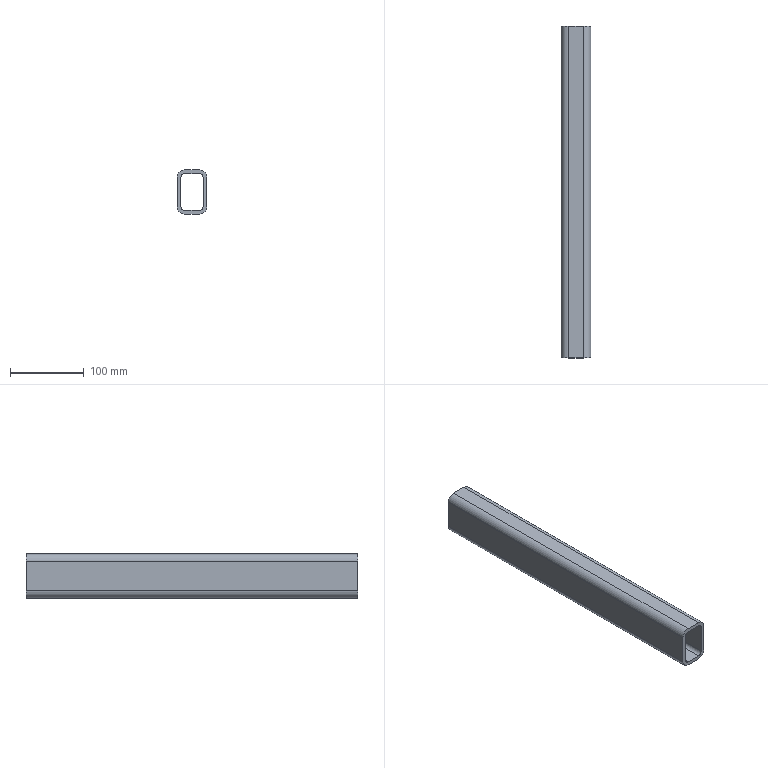Part | STEP file | HL4GD-1.30.110 base frame rear crossmember--20251212 | 1 solid | 18 faces | box 40 x 450 x 60 mm | volume 376029 mm3 | plane 10 | cylinder 8 | commonest cylinder face diameters 10 x4 20 x4
STEP:
#1=CARTESIAN_POINT('',(0.,0.,0.));
#2=DIRECTION('',(0.,0.,1.));
#3=DIRECTION('',(1.,0.,0.));
#4=AXIS2_PLACEMENT_3D('',#1,#2,#3);
#5=CARTESIAN_POINT('',(1525.,1110.,410.));
#6=VERTEX_POINT('',#5);
#7=CARTESIAN_POINT('',(1520.,1110.,415.));
#8=VERTEX_POINT('',#7);
#9=CARTESIAN_POINT('',(1525.,1110.,415.));
#10=DIRECTION('',(0.,1.,0.));
#11=DIRECTION('',(0.,0.,1.));
#12=AXIS2_PLACEMENT_3D('',#9,#10,#11);
#13=CIRCLE('',#12,5.);
#14=CARTESIAN_POINT('',(1525.,530.,415.));
#15=DIRECTION('',(0.,1.,0.));
#16=DIRECTION('',(-1.,0.,0.));
#17=AXIS2_PLACEMENT_3D('',#14,#15,#16);
#18=CYLINDRICAL_SURFACE('',#17,5.);
#19=CARTESIAN_POINT('',(1.571,580.));
#20=DIRECTION('',(1.,0.));
#21=VECTOR('',#20,1.);
#22=LINE('',#19,#21);
#23=(GEOMETRIC_REPRESENTATION_CONTEXT(2)PARAMETRIC_REPRESENTATION_CONTEXT()REPRESENTATION_CONTEXT('',''));
#24=DEFINITIONAL_REPRESENTATION('',(#22),#23);
#25=PCURVE('',#18,#24);
#26=CARTESIAN_POINT('',(2045.,1110.,435.));
#27=DIRECTION('',(0.,1.,0.));
#28=DIRECTION('',(0.,0.,1.));
#29=AXIS2_PLACEMENT_3D('',#26,#27,#28);
#30=PLANE('',#29);
#31=CARTESIAN_POINT('',(-20.,-520.));
#32=DIRECTION('',(1.,0.));
#33=AXIS2_PLACEMENT_2D('',#31,#32);
#34=CIRCLE('',#33,5.);
#35=(GEOMETRIC_REPRESENTATION_CONTEXT(2)PARAMETRIC_REPRESENTATION_CONTEXT()REPRESENTATION_CONTEXT('',''));
#36=DEFINITIONAL_REPRESENTATION('',(#34),#35);
#37=PCURVE('',#30,#36);
#38=SURFACE_CURVE('',#13,(#25,#37),.PCURVE_S1.);
#39=EDGE_CURVE('',#6,#8,#38,.T.);
#40=ORIENTED_EDGE('',*,*,#39,.F.);
#41=CARTESIAN_POINT('',(1525.,660.,410.));
#42=VERTEX_POINT('',#41);
#43=CARTESIAN_POINT('',(1525.,530.,410.));
#44=DIRECTION('',(0.,1.,0.));
#45=VECTOR('',#44,1.);
#46=LINE('',#43,#45);
#47=CARTESIAN_POINT('',(4.712,0.));
#48=DIRECTION('',(0.,1.));
#49=VECTOR('',#48,1.);
#50=LINE('',#47,#49);
#51=(GEOMETRIC_REPRESENTATION_CONTEXT(2)PARAMETRIC_REPRESENTATION_CONTEXT()REPRESENTATION_CONTEXT('',''));
#52=DEFINITIONAL_REPRESENTATION('',(#50),#51);
#53=PCURVE('',#18,#52);
#54=CARTESIAN_POINT('',(1545.,530.,410.));
#55=DIRECTION('',(0.,0.,1.));
#56=DIRECTION('',(1.,0.,0.));
#57=AXIS2_PLACEMENT_3D('',#54,#55,#56);
#58=PLANE('',#57);
#59=CARTESIAN_POINT('',(-20.,0.));
#60=DIRECTION('',(0.,1.));
#61=VECTOR('',#60,1.);
#62=LINE('',#59,#61);
#63=(GEOMETRIC_REPRESENTATION_CONTEXT(2)PARAMETRIC_REPRESENTATION_CONTEXT()REPRESENTATION_CONTEXT('',''));
#64=DEFINITIONAL_REPRESENTATION('',(#62),#63);
#65=PCURVE('',#58,#64);
#66=SURFACE_CURVE('',#46,(#53,#65),.PCURVE_S1.);
#67=EDGE_CURVE('',#42,#6,#66,.T.);
#68=ORIENTED_EDGE('',*,*,#67,.F.);
#69=CARTESIAN_POINT('',(1520.,660.,415.));
#70=VERTEX_POINT('',#69);
#71=CARTESIAN_POINT('',(1525.,660.,415.));
#72=DIRECTION('',(0.,-1.,0.));
#73=DIRECTION('',(0.,0.,-1.));
#74=AXIS2_PLACEMENT_3D('',#71,#72,#73);
#75=CIRCLE('',#74,5.);
#76=CARTESIAN_POINT('',(10.996,130.));
#77=DIRECTION('',(-1.,0.));
#78=VECTOR('',#77,1.);
#79=LINE('',#76,#78);
#80=(GEOMETRIC_REPRESENTATION_CONTEXT(2)PARAMETRIC_REPRESENTATION_CONTEXT()REPRESENTATION_CONTEXT('',''));
#81=DEFINITIONAL_REPRESENTATION('',(#79),#80);
#82=PCURVE('',#18,#81);
#83=CARTESIAN_POINT('',(1555.,660.,412.726));
#84=DIRECTION('',(0.,-1.,0.));
#85=DIRECTION('',(0.,0.,-1.));
#86=AXIS2_PLACEMENT_3D('',#83,#84,#85);
#87=PLANE('',#86);
#88=CARTESIAN_POINT('',(-2.274,-30.));
#89=DIRECTION('',(1.,0.));
#90=AXIS2_PLACEMENT_2D('',#88,#89);
#91=CIRCLE('',#90,5.);
#92=(GEOMETRIC_REPRESENTATION_CONTEXT(2)PARAMETRIC_REPRESENTATION_CONTEXT()REPRESENTATION_CONTEXT('',''));
#93=DEFINITIONAL_REPRESENTATION('',(#91),#92);
#94=PCURVE('',#87,#93);
#95=SURFACE_CURVE('',#75,(#82,#94),.PCURVE_S1.);
#96=EDGE_CURVE('',#70,#42,#95,.T.);
#97=ORIENTED_EDGE('',*,*,#96,.F.);
#98=CARTESIAN_POINT('',(1520.,530.,415.));
#99=DIRECTION('',(0.,1.,0.));
#100=VECTOR('',#99,1.);
#101=LINE('',#98,#100);
#102=CARTESIAN_POINT('',(6.283,0.));
#103=DIRECTION('',(0.,1.));
#104=VECTOR('',#103,1.);
#105=LINE('',#102,#104);
#106=(GEOMETRIC_REPRESENTATION_CONTEXT(2)PARAMETRIC_REPRESENTATION_CONTEXT()REPRESENTATION_CONTEXT('',''));
#107=DEFINITIONAL_REPRESENTATION('',(#105),#106);
#108=PCURVE('',#18,#107);
#109=CARTESIAN_POINT('',(1520.,530.,415.));
#110=DIRECTION('',(1.,0.,0.));
#111=DIRECTION('',(0.,0.,-1.));
#112=AXIS2_PLACEMENT_3D('',#109,#110,#111);
#113=PLANE('',#112);
#114=CARTESIAN_POINT('',(0.,0.));
#115=DIRECTION('',(0.,1.));
#116=VECTOR('',#115,1.);
#117=LINE('',#114,#116);
#118=(GEOMETRIC_REPRESENTATION_CONTEXT(2)PARAMETRIC_REPRESENTATION_CONTEXT()REPRESENTATION_CONTEXT('',''));
#119=DEFINITIONAL_REPRESENTATION('',(#117),#118);
#120=PCURVE('',#113,#119);
#121=SURFACE_CURVE('',#101,(#108,#120),.PCURVE_S1.);
#122=EDGE_CURVE('',#70,#8,#121,.T.);
#123=ORIENTED_EDGE('',*,*,#122,.T.);
#124=EDGE_LOOP('',(#40,#68,#97,#123));
#125=FACE_BOUND('',#124,.F.);
#126=ADVANCED_FACE('',(#125),#18,.F.);
#127=ORIENTED_EDGE('',*,*,#67,.F.);
#128=CARTESIAN_POINT('',(1545.,660.,410.));
#129=VERTEX_POINT('',#128);
#130=CARTESIAN_POINT('',(1545.,660.,410.));
#131=DIRECTION('',(1.,0.,0.));
#132=VECTOR('',#131,1.);
#133=LINE('',#130,#132);
#134=CARTESIAN_POINT('',(0.,130.));
#135=DIRECTION('',(1.,0.));
#136=VECTOR('',#135,1.);
#137=LINE('',#134,#136);
#138=(GEOMETRIC_REPRESENTATION_CONTEXT(2)PARAMETRIC_REPRESENTATION_CONTEXT()REPRESENTATION_CONTEXT('',''));
#139=DEFINITIONAL_REPRESENTATION('',(#137),#138);
#140=PCURVE('',#58,#139);
#141=CARTESIAN_POINT('',(2.726,-10.));
#142=DIRECTION('',(0.,1.));
#143=VECTOR('',#142,1.);
#144=LINE('',#141,#143);
#145=(GEOMETRIC_REPRESENTATION_CONTEXT(2)PARAMETRIC_REPRESENTATION_CONTEXT()REPRESENTATION_CONTEXT('',''));
#146=DEFINITIONAL_REPRESENTATION('',(#144),#145);
#147=PCURVE('',#87,#146);
#148=SURFACE_CURVE('',#133,(#140,#147),.PCURVE_S1.);
#149=EDGE_CURVE('',#42,#129,#148,.T.);
#150=ORIENTED_EDGE('',*,*,#149,.T.);
#151=CARTESIAN_POINT('',(1545.,1110.,410.));
#152=VERTEX_POINT('',#151);
#153=CARTESIAN_POINT('',(1545.,530.,410.));
#154=DIRECTION('',(0.,1.,0.));
#155=VECTOR('',#154,1.);
#156=LINE('',#153,#155);
#157=CARTESIAN_POINT('',(0.,0.));
#158=DIRECTION('',(0.,1.));
#159=VECTOR('',#158,1.);
#160=LINE('',#157,#159);
#161=(GEOMETRIC_REPRESENTATION_CONTEXT(2)PARAMETRIC_REPRESENTATION_CONTEXT()REPRESENTATION_CONTEXT('',''));
#162=DEFINITIONAL_REPRESENTATION('',(#160),#161);
#163=PCURVE('',#58,#162);
#164=CARTESIAN_POINT('',(1545.,530.,415.));
#165=DIRECTION('',(0.,1.,0.));
#166=DIRECTION('',(-1.,0.,0.));
#167=AXIS2_PLACEMENT_3D('',#164,#165,#166);
#168=CYLINDRICAL_SURFACE('',#167,5.);
#169=CARTESIAN_POINT('',(4.712,0.));
#170=DIRECTION('',(0.,1.));
#171=VECTOR('',#170,1.);
#172=LINE('',#169,#171);
#173=(GEOMETRIC_REPRESENTATION_CONTEXT(2)PARAMETRIC_REPRESENTATION_CONTEXT()REPRESENTATION_CONTEXT('',''));
#174=DEFINITIONAL_REPRESENTATION('',(#172),#173);
#175=PCURVE('',#168,#174);
#176=SURFACE_CURVE('',#156,(#163,#175),.PCURVE_S1.);
#177=EDGE_CURVE('',#129,#152,#176,.T.);
#178=ORIENTED_EDGE('',*,*,#177,.T.);
#179=CARTESIAN_POINT('',(1545.,1110.,410.));
#180=DIRECTION('',(-1.,0.,0.));
#181=VECTOR('',#180,1.);
#182=LINE('',#179,#181);
#183=CARTESIAN_POINT('',(0.,580.));
#184=DIRECTION('',(-1.,0.));
#185=VECTOR('',#184,1.);
#186=LINE('',#183,#185);
#187=(GEOMETRIC_REPRESENTATION_CONTEXT(2)PARAMETRIC_REPRESENTATION_CONTEXT()REPRESENTATION_CONTEXT('',''));
#188=DEFINITIONAL_REPRESENTATION('',(#186),#187);
#189=PCURVE('',#58,#188);
#190=CARTESIAN_POINT('',(-25.,-500.));
#191=DIRECTION('',(0.,-1.));
#192=VECTOR('',#191,1.);
#193=LINE('',#190,#192);
#194=(GEOMETRIC_REPRESENTATION_CONTEXT(2)PARAMETRIC_REPRESENTATION_CONTEXT()REPRESENTATION_CONTEXT('',''));
#195=DEFINITIONAL_REPRESENTATION('',(#193),#194);
#196=PCURVE('',#30,#195);
#197=SURFACE_CURVE('',#182,(#189,#196),.PCURVE_S1.);
#198=EDGE_CURVE('',#152,#6,#197,.T.);
#199=ORIENTED_EDGE('',*,*,#198,.T.);
#200=EDGE_LOOP('',(#127,#150,#178,#199));
#201=FACE_BOUND('',#200,.T.);
#202=ADVANCED_FACE('',(#201),#58,.T.);
#203=CARTESIAN_POINT('',(1550.,1110.,415.));
#204=VERTEX_POINT('',#203);
#205=CARTESIAN_POINT('',(1545.,1110.,415.));
#206=DIRECTION('',(0.,1.,0.));
#207=DIRECTION('',(0.,0.,1.));
#208=AXIS2_PLACEMENT_3D('',#205,#206,#207);
#209=CIRCLE('',#208,5.);
#210=CARTESIAN_POINT('',(1.571,580.));
#211=DIRECTION('',(1.,0.));
#212=VECTOR('',#211,1.);
#213=LINE('',#210,#212);
#214=(GEOMETRIC_REPRESENTATION_CONTEXT(2)PARAMETRIC_REPRESENTATION_CONTEXT()REPRESENTATION_CONTEXT('',''));
#215=DEFINITIONAL_REPRESENTATION('',(#213),#214);
#216=PCURVE('',#168,#215);
#217=CARTESIAN_POINT('',(-20.,-500.));
#218=DIRECTION('',(1.,0.));
#219=AXIS2_PLACEMENT_2D('',#217,#218);
#220=CIRCLE('',#219,5.);
#221=(GEOMETRIC_REPRESENTATION_CONTEXT(2)PARAMETRIC_REPRESENTATION_CONTEXT()REPRESENTATION_CONTEXT('',''));
#222=DEFINITIONAL_REPRESENTATION('',(#220),#221);
#223=PCURVE('',#30,#222);
#224=SURFACE_CURVE('',#209,(#216,#223),.PCURVE_S1.);
#225=EDGE_CURVE('',#204,#152,#224,.T.);
#226=ORIENTED_EDGE('',*,*,#225,.F.);
#227=CARTESIAN_POINT('',(1550.,660.,415.));
#228=VERTEX_POINT('',#227);
#229=CARTESIAN_POINT('',(1550.,530.,415.));
#230=DIRECTION('',(0.,1.,0.));
#231=VECTOR('',#230,1.);
#232=LINE('',#229,#231);
#233=CARTESIAN_POINT('',(3.142,0.));
#234=DIRECTION('',(0.,1.));
#235=VECTOR('',#234,1.);
#236=LINE('',#233,#235);
#237=(GEOMETRIC_REPRESENTATION_CONTEXT(2)PARAMETRIC_REPRESENTATION_CONTEXT()REPRESENTATION_CONTEXT('',''));
#238=DEFINITIONAL_REPRESENTATION('',(#236),#237);
#239=PCURVE('',#168,#238);
#240=CARTESIAN_POINT('',(1550.,530.,455.));
#241=DIRECTION('',(-1.,0.,0.));
#242=DIRECTION('',(0.,0.,1.));
#243=AXIS2_PLACEMENT_3D('',#240,#241,#242);
#244=PLANE('',#243);
#245=CARTESIAN_POINT('',(-40.,0.));
#246=DIRECTION('',(0.,1.));
#247=VECTOR('',#246,1.);
#248=LINE('',#245,#247);
#249=(GEOMETRIC_REPRESENTATION_CONTEXT(2)PARAMETRIC_REPRESENTATION_CONTEXT()REPRESENTATION_CONTEXT('',''));
#250=DEFINITIONAL_REPRESENTATION('',(#248),#249);
#251=PCURVE('',#244,#250);
#252=SURFACE_CURVE('',#232,(#239,#251),.PCURVE_S1.);
#253=EDGE_CURVE('',#228,#204,#252,.T.);
#254=ORIENTED_EDGE('',*,*,#253,.F.);
#255=CARTESIAN_POINT('',(1545.,660.,415.));
#256=DIRECTION('',(0.,-1.,0.));
#257=DIRECTION('',(0.,0.,-1.));
#258=AXIS2_PLACEMENT_3D('',#255,#256,#257);
#259=CIRCLE('',#258,5.);
#260=CARTESIAN_POINT('',(4.712,130.));
#261=DIRECTION('',(-1.,0.));
#262=VECTOR('',#261,1.);
#263=LINE('',#260,#262);
#264=(GEOMETRIC_REPRESENTATION_CONTEXT(2)PARAMETRIC_REPRESENTATION_CONTEXT()REPRESENTATION_CONTEXT('',''));
#265=DEFINITIONAL_REPRESENTATION('',(#263),#264);
#266=PCURVE('',#168,#265);
#267=CARTESIAN_POINT('',(-2.274,-10.));
#268=DIRECTION('',(1.,0.));
#269=AXIS2_PLACEMENT_2D('',#267,#268);
#270=CIRCLE('',#269,5.);
#271=(GEOMETRIC_REPRESENTATION_CONTEXT(2)PARAMETRIC_REPRESENTATION_CONTEXT()REPRESENTATION_CONTEXT('',''));
#272=DEFINITIONAL_REPRESENTATION('',(#270),#271);
#273=PCURVE('',#87,#272);
#274=SURFACE_CURVE('',#259,(#266,#273),.PCURVE_S1.);
#275=EDGE_CURVE('',#129,#228,#274,.T.);
#276=ORIENTED_EDGE('',*,*,#275,.F.);
#277=ORIENTED_EDGE('',*,*,#177,.T.);
#278=EDGE_LOOP('',(#226,#254,#276,#277));
#279=FACE_BOUND('',#278,.F.);
#280=ADVANCED_FACE('',(#279),#168,.F.);
#281=ORIENTED_EDGE('',*,*,#253,.F.);
#282=CARTESIAN_POINT('',(1550.,660.,455.));
#283=VERTEX_POINT('',#282);
#284=CARTESIAN_POINT('',(1550.,660.,455.));
#285=DIRECTION('',(0.,0.,1.));
#286=VECTOR('',#285,1.);
#287=LINE('',#284,#286);
#288=CARTESIAN_POINT('',(0.,130.));
#289=DIRECTION('',(1.,0.));
#290=VECTOR('',#289,1.);
#291=LINE('',#288,#290);
#292=(GEOMETRIC_REPRESENTATION_CONTEXT(2)PARAMETRIC_REPRESENTATION_CONTEXT()REPRESENTATION_CONTEXT('',''));
#293=DEFINITIONAL_REPRESENTATION('',(#291),#292);
#294=PCURVE('',#244,#293);
#295=CARTESIAN_POINT('',(-42.274,-5.));
#296=DIRECTION('',(-1.,0.));
#297=VECTOR('',#296,1.);
#298=LINE('',#295,#297);
#299=(GEOMETRIC_REPRESENTATION_CONTEXT(2)PARAMETRIC_REPRESENTATION_CONTEXT()REPRESENTATION_CONTEXT('',''));
#300=DEFINITIONAL_REPRESENTATION('',(#298),#299);
#301=PCURVE('',#87,#300);
#302=SURFACE_CURVE('',#287,(#294,#301),.PCURVE_S1.);
#303=EDGE_CURVE('',#228,#283,#302,.T.);
#304=ORIENTED_EDGE('',*,*,#303,.T.);
#305=CARTESIAN_POINT('',(1550.,1110.,455.));
#306=VERTEX_POINT('',#305);
#307=CARTESIAN_POINT('',(1550.,530.,455.));
#308=DIRECTION('',(0.,1.,0.));
#309=VECTOR('',#308,1.);
#310=LINE('',#307,#309);
#311=CARTESIAN_POINT('',(0.,0.));
#312=DIRECTION('',(0.,1.));
#313=VECTOR('',#312,1.);
#314=LINE('',#311,#313);
#315=(GEOMETRIC_REPRESENTATION_CONTEXT(2)PARAMETRIC_REPRESENTATION_CONTEXT()REPRESENTATION_CONTEXT('',''));
#316=DEFINITIONAL_REPRESENTATION('',(#314),#315);
#317=PCURVE('',#244,#316);
#318=CARTESIAN_POINT('',(1545.,530.,455.));
#319=DIRECTION('',(0.,1.,0.));
#320=DIRECTION('',(-1.,0.,0.));
#321=AXIS2_PLACEMENT_3D('',#318,#319,#320);
#322=CYLINDRICAL_SURFACE('',#321,5.);
#323=CARTESIAN_POINT('',(3.142,0.));
#324=DIRECTION('',(0.,1.));
#325=VECTOR('',#324,1.);
#326=LINE('',#323,#325);
#327=(GEOMETRIC_REPRESENTATION_CONTEXT(2)PARAMETRIC_REPRESENTATION_CONTEXT()REPRESENTATION_CONTEXT('',''));
#328=DEFINITIONAL_REPRESENTATION('',(#326),#327);
#329=PCURVE('',#322,#328);
#330=SURFACE_CURVE('',#310,(#317,#329),.PCURVE_S1.);
#331=EDGE_CURVE('',#283,#306,#330,.T.);
#332=ORIENTED_EDGE('',*,*,#331,.T.);
#333=CARTESIAN_POINT('',(1550.,1110.,455.));
#334=DIRECTION('',(0.,0.,-1.));
#335=VECTOR('',#334,1.);
#336=LINE('',#333,#335);
#337=CARTESIAN_POINT('',(0.,580.));
#338=DIRECTION('',(-1.,0.));
#339=VECTOR('',#338,1.);
#340=LINE('',#337,#339);
#341=(GEOMETRIC_REPRESENTATION_CONTEXT(2)PARAMETRIC_REPRESENTATION_CONTEXT()REPRESENTATION_CONTEXT('',''));
#342=DEFINITIONAL_REPRESENTATION('',(#340),#341);
#343=PCURVE('',#244,#342);
#344=CARTESIAN_POINT('',(20.,-495.));
#345=DIRECTION('',(-1.,0.));
#346=VECTOR('',#345,1.);
#347=LINE('',#344,#346);
#348=(GEOMETRIC_REPRESENTATION_CONTEXT(2)PARAMETRIC_REPRESENTATION_CONTEXT()REPRESENTATION_CONTEXT('',''));
#349=DEFINITIONAL_REPRESENTATION('',(#347),#348);
#350=PCURVE('',#30,#349);
#351=SURFACE_CURVE('',#336,(#343,#350),.PCURVE_S1.);
#352=EDGE_CURVE('',#306,#204,#351,.T.);
#353=ORIENTED_EDGE('',*,*,#352,.T.);
#354=EDGE_LOOP('',(#281,#304,#332,#353));
#355=FACE_BOUND('',#354,.T.);
#356=ADVANCED_FACE('',(#355),#244,.T.);
#357=CARTESIAN_POINT('',(1545.,1110.,460.));
#358=VERTEX_POINT('',#357);
#359=CARTESIAN_POINT('',(1545.,1110.,455.));
#360=DIRECTION('',(0.,1.,0.));
#361=DIRECTION('',(0.,0.,1.));
#362=AXIS2_PLACEMENT_3D('',#359,#360,#361);
#363=CIRCLE('',#362,5.);
#364=CARTESIAN_POINT('',(1.571,580.));
#365=DIRECTION('',(1.,0.));
#366=VECTOR('',#365,1.);
#367=LINE('',#364,#366);
#368=(GEOMETRIC_REPRESENTATION_CONTEXT(2)PARAMETRIC_REPRESENTATION_CONTEXT()REPRESENTATION_CONTEXT('',''));
#369=DEFINITIONAL_REPRESENTATION('',(#367),#368);
#370=PCURVE('',#322,#369);
#371=CARTESIAN_POINT('',(20.,-500.));
#372=DIRECTION('',(1.,0.));
#373=AXIS2_PLACEMENT_2D('',#371,#372);
#374=CIRCLE('',#373,5.);
#375=(GEOMETRIC_REPRESENTATION_CONTEXT(2)PARAMETRIC_REPRESENTATION_CONTEXT()REPRESENTATION_CONTEXT('',''));
#376=DEFINITIONAL_REPRESENTATION('',(#374),#375);
#377=PCURVE('',#30,#376);
#378=SURFACE_CURVE('',#363,(#370,#377),.PCURVE_S1.);
#379=EDGE_CURVE('',#358,#306,#378,.T.);
#380=ORIENTED_EDGE('',*,*,#379,.F.);
#381=CARTESIAN_POINT('',(1545.,660.,460.));
#382=VERTEX_POINT('',#381);
#383=CARTESIAN_POINT('',(1545.,530.,460.));
#384=DIRECTION('',(0.,1.,0.));
#385=VECTOR('',#384,1.);
#386=LINE('',#383,#385);
#387=CARTESIAN_POINT('',(1.571,0.));
#388=DIRECTION('',(0.,1.));
#389=VECTOR('',#388,1.);
#390=LINE('',#387,#389);
#391=(GEOMETRIC_REPRESENTATION_CONTEXT(2)PARAMETRIC_REPRESENTATION_CONTEXT()REPRESENTATION_CONTEXT('',''));
#392=DEFINITIONAL_REPRESENTATION('',(#390),#391);
#393=PCURVE('',#322,#392);
#394=CARTESIAN_POINT('',(1525.,530.,460.));
#395=DIRECTION('',(0.,0.,-1.));
#396=DIRECTION('',(-1.,0.,0.));
#397=AXIS2_PLACEMENT_3D('',#394,#395,#396);
#398=PLANE('',#397);
#399=CARTESIAN_POINT('',(-20.,0.));
#400=DIRECTION('',(0.,1.));
#401=VECTOR('',#400,1.);
#402=LINE('',#399,#401);
#403=(GEOMETRIC_REPRESENTATION_CONTEXT(2)PARAMETRIC_REPRESENTATION_CONTEXT()REPRESENTATION_CONTEXT('',''));
#404=DEFINITIONAL_REPRESENTATION('',(#402),#403);
#405=PCURVE('',#398,#404);
#406=SURFACE_CURVE('',#386,(#393,#405),.PCURVE_S1.);
#407=EDGE_CURVE('',#382,#358,#406,.T.);
#408=ORIENTED_EDGE('',*,*,#407,.F.);
#409=CARTESIAN_POINT('',(1545.,660.,455.));
#410=DIRECTION('',(0.,-1.,0.));
#411=DIRECTION('',(0.,0.,-1.));
#412=AXIS2_PLACEMENT_3D('',#409,#410,#411);
#413=CIRCLE('',#412,5.);
#414=CARTESIAN_POINT('',(4.712,130.));
#415=DIRECTION('',(-1.,0.));
#416=VECTOR('',#415,1.);
#417=LINE('',#414,#416);
#418=(GEOMETRIC_REPRESENTATION_CONTEXT(2)PARAMETRIC_REPRESENTATION_CONTEXT()REPRESENTATION_CONTEXT('',''));
#419=DEFINITIONAL_REPRESENTATION('',(#417),#418);
#420=PCURVE('',#322,#419);
#421=CARTESIAN_POINT('',(-42.274,-10.));
#422=DIRECTION('',(1.,0.));
#423=AXIS2_PLACEMENT_2D('',#421,#422);
#424=CIRCLE('',#423,5.);
#425=(GEOMETRIC_REPRESENTATION_CONTEXT(2)PARAMETRIC_REPRESENTATION_CONTEXT()REPRESENTATION_CONTEXT('',''));
#426=DEFINITIONAL_REPRESENTATION('',(#424),#425);
#427=PCURVE('',#87,#426);
#428=SURFACE_CURVE('',#413,(#420,#427),.PCURVE_S1.);
#429=EDGE_CURVE('',#283,#382,#428,.T.);
#430=ORIENTED_EDGE('',*,*,#429,.F.);
#431=ORIENTED_EDGE('',*,*,#331,.T.);
#432=EDGE_LOOP('',(#380,#408,#430,#431));
#433=FACE_BOUND('',#432,.F.);
#434=ADVANCED_FACE('',(#433),#322,.F.);
#435=ORIENTED_EDGE('',*,*,#407,.F.);
#436=CARTESIAN_POINT('',(1525.,660.,460.));
#437=VERTEX_POINT('',#436);
#438=CARTESIAN_POINT('',(1525.,660.,460.));
#439=DIRECTION('',(-1.,0.,0.));
#440=VECTOR('',#439,1.);
#441=LINE('',#438,#440);
#442=CARTESIAN_POINT('',(0.,130.));
#443=DIRECTION('',(1.,0.));
#444=VECTOR('',#443,1.);
#445=LINE('',#442,#444);
#446=(GEOMETRIC_REPRESENTATION_CONTEXT(2)PARAMETRIC_REPRESENTATION_CONTEXT()REPRESENTATION_CONTEXT('',''));
#447=DEFINITIONAL_REPRESENTATION('',(#445),#446);
#448=PCURVE('',#398,#447);
#449=CARTESIAN_POINT('',(-47.274,-30.));
#450=DIRECTION('',(0.,-1.));
#451=VECTOR('',#450,1.);
#452=LINE('',#449,#451);
#453=(GEOMETRIC_REPRESENTATION_CONTEXT(2)PARAMETRIC_REPRESENTATION_CONTEXT()REPRESENTATION_CONTEXT('',''));
#454=DEFINITIONAL_REPRESENTATION('',(#452),#453);
#455=PCURVE('',#87,#454);
#456=SURFACE_CURVE('',#441,(#448,#455),.PCURVE_S1.);
#457=EDGE_CURVE('',#382,#437,#456,.T.);
#458=ORIENTED_EDGE('',*,*,#457,.T.);
#459=CARTESIAN_POINT('',(1525.,1110.,460.));
#460=VERTEX_POINT('',#459);
#461=CARTESIAN_POINT('',(1525.,530.,460.));
#462=DIRECTION('',(0.,1.,0.));
#463=VECTOR('',#462,1.);
#464=LINE('',#461,#463);
#465=CARTESIAN_POINT('',(0.,0.));
#466=DIRECTION('',(0.,1.));
#467=VECTOR('',#466,1.);
#468=LINE('',#465,#467);
#469=(GEOMETRIC_REPRESENTATION_CONTEXT(2)PARAMETRIC_REPRESENTATION_CONTEXT()REPRESENTATION_CONTEXT('',''));
#470=DEFINITIONAL_REPRESENTATION('',(#468),#469);
#471=PCURVE('',#398,#470);
#472=CARTESIAN_POINT('',(1525.,530.,455.));
#473=DIRECTION('',(0.,1.,0.));
#474=DIRECTION('',(-1.,0.,0.));
#475=AXIS2_PLACEMENT_3D('',#472,#473,#474);
#476=CYLINDRICAL_SURFACE('',#475,5.);
#477=CARTESIAN_POINT('',(1.571,0.));
#478=DIRECTION('',(0.,1.));
#479=VECTOR('',#478,1.);
#480=LINE('',#477,#479);
#481=(GEOMETRIC_REPRESENTATION_CONTEXT(2)PARAMETRIC_REPRESENTATION_CONTEXT()REPRESENTATION_CONTEXT('',''));
#482=DEFINITIONAL_REPRESENTATION('',(#480),#481);
#483=PCURVE('',#476,#482);
#484=SURFACE_CURVE('',#464,(#471,#483),.PCURVE_S1.);
#485=EDGE_CURVE('',#437,#460,#484,.T.);
#486=ORIENTED_EDGE('',*,*,#485,.T.);
#487=CARTESIAN_POINT('',(1525.,1110.,460.));
#488=DIRECTION('',(1.,0.,0.));
#489=VECTOR('',#488,1.);
#490=LINE('',#487,#489);
#491=CARTESIAN_POINT('',(0.,580.));
#492=DIRECTION('',(-1.,0.));
#493=VECTOR('',#492,1.);
#494=LINE('',#491,#493);
#495=(GEOMETRIC_REPRESENTATION_CONTEXT(2)PARAMETRIC_REPRESENTATION_CONTEXT()REPRESENTATION_CONTEXT('',''));
#496=DEFINITIONAL_REPRESENTATION('',(#494),#495);
#497=PCURVE('',#398,#496);
#498=CARTESIAN_POINT('',(25.,-520.));
#499=DIRECTION('',(0.,1.));
#500=VECTOR('',#499,1.);
#501=LINE('',#498,#500);
#502=(GEOMETRIC_REPRESENTATION_CONTEXT(2)PARAMETRIC_REPRESENTATION_CONTEXT()REPRESENTATION_CONTEXT('',''));
#503=DEFINITIONAL_REPRESENTATION('',(#501),#502);
#504=PCURVE('',#30,#503);
#505=SURFACE_CURVE('',#490,(#497,#504),.PCURVE_S1.);
#506=EDGE_CURVE('',#460,#358,#505,.T.);
#507=ORIENTED_EDGE('',*,*,#506,.T.);
#508=EDGE_LOOP('',(#435,#458,#486,#507));
#509=FACE_BOUND('',#508,.T.);
#510=ADVANCED_FACE('',(#509),#398,.T.);
#511=CARTESIAN_POINT('',(1520.,1110.,455.));
#512=VERTEX_POINT('',#511);
#513=CARTESIAN_POINT('',(1525.,1110.,455.));
#514=DIRECTION('',(0.,1.,0.));
#515=DIRECTION('',(0.,0.,1.));
#516=AXIS2_PLACEMENT_3D('',#513,#514,#515);
#517=CIRCLE('',#516,5.);
#518=CARTESIAN_POINT('',(-4.712,580.));
#519=DIRECTION('',(1.,0.));
#520=VECTOR('',#519,1.);
#521=LINE('',#518,#520);
#522=(GEOMETRIC_REPRESENTATION_CONTEXT(2)PARAMETRIC_REPRESENTATION_CONTEXT()REPRESENTATION_CONTEXT('',''));
#523=DEFINITIONAL_REPRESENTATION('',(#521),#522);
#524=PCURVE('',#476,#523);
#525=CARTESIAN_POINT('',(20.,-520.));
#526=DIRECTION('',(1.,0.));
#527=AXIS2_PLACEMENT_2D('',#525,#526);
#528=CIRCLE('',#527,5.);
#529=(GEOMETRIC_REPRESENTATION_CONTEXT(2)PARAMETRIC_REPRESENTATION_CONTEXT()REPRESENTATION_CONTEXT('',''));
#530=DEFINITIONAL_REPRESENTATION('',(#528),#529);
#531=PCURVE('',#30,#530);
#532=SURFACE_CURVE('',#517,(#524,#531),.PCURVE_S1.);
#533=EDGE_CURVE('',#512,#460,#532,.T.);
#534=ORIENTED_EDGE('',*,*,#533,.F.);
#535=CARTESIAN_POINT('',(1520.,660.,455.));
#536=VERTEX_POINT('',#535);
#537=CARTESIAN_POINT('',(1520.,530.,455.));
#538=DIRECTION('',(0.,1.,0.));
#539=VECTOR('',#538,1.);
#540=LINE('',#537,#539);
#541=CARTESIAN_POINT('',(0.,0.));
#542=DIRECTION('',(0.,1.));
#543=VECTOR('',#542,1.);
#544=LINE('',#541,#543);
#545=(GEOMETRIC_REPRESENTATION_CONTEXT(2)PARAMETRIC_REPRESENTATION_CONTEXT()REPRESENTATION_CONTEXT('',''));
#546=DEFINITIONAL_REPRESENTATION('',(#544),#545);
#547=PCURVE('',#476,#546);
#548=CARTESIAN_POINT('',(-40.,0.));
#549=DIRECTION('',(0.,1.));
#550=VECTOR('',#549,1.);
#551=LINE('',#548,#550);
#552=(GEOMETRIC_REPRESENTATION_CONTEXT(2)PARAMETRIC_REPRESENTATION_CONTEXT()REPRESENTATION_CONTEXT('',''));
#553=DEFINITIONAL_REPRESENTATION('',(#551),#552);
#554=PCURVE('',#113,#553);
#555=SURFACE_CURVE('',#540,(#547,#554),.PCURVE_S1.);
#556=EDGE_CURVE('',#536,#512,#555,.T.);
#557=ORIENTED_EDGE('',*,*,#556,.F.);
#558=CARTESIAN_POINT('',(1525.,660.,455.));
#559=DIRECTION('',(0.,-1.,0.));
#560=DIRECTION('',(0.,0.,-1.));
#561=AXIS2_PLACEMENT_3D('',#558,#559,#560);
#562=CIRCLE('',#561,5.);
#563=CARTESIAN_POINT('',(4.712,130.));
#564=DIRECTION('',(-1.,0.));
#565=VECTOR('',#564,1.);
#566=LINE('',#563,#565);
#567=(GEOMETRIC_REPRESENTATION_CONTEXT(2)PARAMETRIC_REPRESENTATION_CONTEXT()REPRESENTATION_CONTEXT('',''));
#568=DEFINITIONAL_REPRESENTATION('',(#566),#567);
#569=PCURVE('',#476,#568);
#570=CARTESIAN_POINT('',(-42.274,-30.));
#571=DIRECTION('',(1.,0.));
#572=AXIS2_PLACEMENT_2D('',#570,#571);
#573=CIRCLE('',#572,5.);
#574=(GEOMETRIC_REPRESENTATION_CONTEXT(2)PARAMETRIC_REPRESENTATION_CONTEXT()REPRESENTATION_CONTEXT('',''));
#575=DEFINITIONAL_REPRESENTATION('',(#573),#574);
#576=PCURVE('',#87,#575);
#577=SURFACE_CURVE('',#562,(#569,#576),.PCURVE_S1.);
#578=EDGE_CURVE('',#437,#536,#577,.T.);
#579=ORIENTED_EDGE('',*,*,#578,.F.);
#580=ORIENTED_EDGE('',*,*,#485,.T.);
#581=EDGE_LOOP('',(#534,#557,#579,#580));
#582=FACE_BOUND('',#581,.F.);
#583=ADVANCED_FACE('',(#582),#476,.F.);
#584=CARTESIAN_POINT('',(1555.,660.,455.));
#585=VERTEX_POINT('',#584);
#586=CARTESIAN_POINT('',(1555.,1110.,455.));
#587=VERTEX_POINT('',#586);
#588=CARTESIAN_POINT('',(1555.,530.,455.));
#589=DIRECTION('',(0.,1.,0.));
#590=VECTOR('',#589,1.);
#591=LINE('',#588,#590);
#592=CARTESIAN_POINT('',(1555.,530.,455.));
#593=DIRECTION('',(-1.,0.,0.));
#594=DIRECTION('',(0.,0.,1.));
#595=AXIS2_PLACEMENT_3D('',#592,#593,#594);
#596=PLANE('',#595);
#597=CARTESIAN_POINT('',(0.,0.));
#598=DIRECTION('',(0.,1.));
#599=VECTOR('',#598,1.);
#600=LINE('',#597,#599);
#601=(GEOMETRIC_REPRESENTATION_CONTEXT(2)PARAMETRIC_REPRESENTATION_CONTEXT()REPRESENTATION_CONTEXT('',''));
#602=DEFINITIONAL_REPRESENTATION('',(#600),#601);
#603=PCURVE('',#596,#602);
#604=CARTESIAN_POINT('',(1545.,530.,455.));
#605=DIRECTION('',(0.,1.,0.));
#606=DIRECTION('',(-1.,0.,0.));
#607=AXIS2_PLACEMENT_3D('',#604,#605,#606);
#608=CYLINDRICAL_SURFACE('',#607,10.);
#609=CARTESIAN_POINT('',(3.142,0.));
#610=DIRECTION('',(0.,1.));
#611=VECTOR('',#610,1.);
#612=LINE('',#609,#611);
#613=(GEOMETRIC_REPRESENTATION_CONTEXT(2)PARAMETRIC_REPRESENTATION_CONTEXT()REPRESENTATION_CONTEXT('',''));
#614=DEFINITIONAL_REPRESENTATION('',(#612),#613);
#615=PCURVE('',#608,#614);
#616=SURFACE_CURVE('',#591,(#603,#615),.PCURVE_S1.);
#617=EDGE_CURVE('',#585,#587,#616,.T.);
#618=ORIENTED_EDGE('',*,*,#617,.F.);
#619=CARTESIAN_POINT('',(1555.,660.,415.));
#620=VERTEX_POINT('',#619);
#621=CARTESIAN_POINT('',(1555.,660.,455.));
#622=DIRECTION('',(0.,0.,-1.));
#623=VECTOR('',#622,1.);
#624=LINE('',#621,#623);
#625=CARTESIAN_POINT('',(0.,130.));
#626=DIRECTION('',(-1.,0.));
#627=VECTOR('',#626,1.);
#628=LINE('',#625,#627);
#629=(GEOMETRIC_REPRESENTATION_CONTEXT(2)PARAMETRIC_REPRESENTATION_CONTEXT()REPRESENTATION_CONTEXT('',''));
#630=DEFINITIONAL_REPRESENTATION('',(#628),#629);
#631=PCURVE('',#596,#630);
#632=CARTESIAN_POINT('',(-42.274,0.));
#633=DIRECTION('',(1.,0.));
#634=VECTOR('',#633,1.);
#635=LINE('',#632,#634);
#636=(GEOMETRIC_REPRESENTATION_CONTEXT(2)PARAMETRIC_REPRESENTATION_CONTEXT()REPRESENTATION_CONTEXT('',''));
#637=DEFINITIONAL_REPRESENTATION('',(#635),#636);
#638=PCURVE('',#87,#637);
#639=SURFACE_CURVE('',#624,(#631,#638),.PCURVE_S1.);
#640=EDGE_CURVE('',#585,#620,#639,.T.);
#641=ORIENTED_EDGE('',*,*,#640,.T.);
#642=CARTESIAN_POINT('',(1555.,1110.,415.));
#643=VERTEX_POINT('',#642);
#644=CARTESIAN_POINT('',(1555.,530.,415.));
#645=DIRECTION('',(0.,1.,0.));
#646=VECTOR('',#645,1.);
#647=LINE('',#644,#646);
#648=CARTESIAN_POINT('',(-40.,0.));
#649=DIRECTION('',(0.,1.));
#650=VECTOR('',#649,1.);
#651=LINE('',#648,#650);
#652=(GEOMETRIC_REPRESENTATION_CONTEXT(2)PARAMETRIC_REPRESENTATION_CONTEXT()REPRESENTATION_CONTEXT('',''));
#653=DEFINITIONAL_REPRESENTATION('',(#651),#652);
#654=PCURVE('',#596,#653);
#655=CARTESIAN_POINT('',(1545.,530.,415.));
#656=DIRECTION('',(0.,1.,0.));
#657=DIRECTION('',(-1.,0.,0.));
#658=AXIS2_PLACEMENT_3D('',#655,#656,#657);
#659=CYLINDRICAL_SURFACE('',#658,10.);
#660=CARTESIAN_POINT('',(3.142,0.));
#661=DIRECTION('',(0.,1.));
#662=VECTOR('',#661,1.);
#663=LINE('',#660,#662);
#664=(GEOMETRIC_REPRESENTATION_CONTEXT(2)PARAMETRIC_REPRESENTATION_CONTEXT()REPRESENTATION_CONTEXT('',''));
#665=DEFINITIONAL_REPRESENTATION('',(#663),#664);
#666=PCURVE('',#659,#665);
#667=SURFACE_CURVE('',#647,(#654,#666),.PCURVE_S1.);
#668=EDGE_CURVE('',#620,#643,#667,.T.);
#669=ORIENTED_EDGE('',*,*,#668,.T.);
#670=CARTESIAN_POINT('',(1555.,1110.,455.));
#671=DIRECTION('',(0.,0.,1.));
#672=VECTOR('',#671,1.);
#673=LINE('',#670,#672);
#674=CARTESIAN_POINT('',(0.,580.));
#675=DIRECTION('',(1.,0.));
#676=VECTOR('',#675,1.);
#677=LINE('',#674,#676);
#678=(GEOMETRIC_REPRESENTATION_CONTEXT(2)PARAMETRIC_REPRESENTATION_CONTEXT()REPRESENTATION_CONTEXT('',''));
#679=DEFINITIONAL_REPRESENTATION('',(#677),#678);
#680=PCURVE('',#596,#679);
#681=CARTESIAN_POINT('',(20.,-490.));
#682=DIRECTION('',(1.,0.));
#683=VECTOR('',#682,1.);
#684=LINE('',#681,#683);
#685=(GEOMETRIC_REPRESENTATION_CONTEXT(2)PARAMETRIC_REPRESENTATION_CONTEXT()REPRESENTATION_CONTEXT('',''));
#686=DEFINITIONAL_REPRESENTATION('',(#684),#685);
#687=PCURVE('',#30,#686);
#688=SURFACE_CURVE('',#673,(#680,#687),.PCURVE_S1.);
#689=EDGE_CURVE('',#643,#587,#688,.T.);
#690=ORIENTED_EDGE('',*,*,#689,.T.);
#691=EDGE_LOOP('',(#618,#641,#669,#690));
#692=FACE_BOUND('',#691,.T.);
#693=ADVANCED_FACE('',(#692),#596,.F.);
#694=ORIENTED_EDGE('',*,*,#668,.F.);
#695=CARTESIAN_POINT('',(1545.,660.,405.));
#696=VERTEX_POINT('',#695);
#697=CARTESIAN_POINT('',(1545.,660.,415.));
#698=DIRECTION('',(0.,1.,0.));
#699=DIRECTION('',(0.,0.,-1.));
#700=AXIS2_PLACEMENT_3D('',#697,#698,#699);
#701=CIRCLE('',#700,10.);
#702=CARTESIAN_POINT('',(-1.571,130.));
#703=DIRECTION('',(1.,0.));
#704=VECTOR('',#703,1.);
#705=LINE('',#702,#704);
#706=(GEOMETRIC_REPRESENTATION_CONTEXT(2)PARAMETRIC_REPRESENTATION_CONTEXT()REPRESENTATION_CONTEXT('',''));
#707=DEFINITIONAL_REPRESENTATION('',(#705),#706);
#708=PCURVE('',#659,#707);
#709=CARTESIAN_POINT('',(7.726,-10.));
#710=CARTESIAN_POINT('',(7.726,-27.321));
#711=CARTESIAN_POINT('',(-7.274,-18.66));
#712=CARTESIAN_POINT('',(-22.274,-10.));
#713=CARTESIAN_POINT('',(-7.274,-1.34));
#714=CARTESIAN_POINT('',(7.726,7.321));
#715=CARTESIAN_POINT('',(7.726,-10.));
#716=(BOUNDED_CURVE()B_SPLINE_CURVE(2,(#709,#710,#711,#712,#713,#714,#715),.UNSPECIFIED.,.T.,.F.)B_SPLINE_CURVE_WITH_KNOTS((1,2,2,2,2,1),(-2.094,0.,2.094,4.189,6.283,8.378),.UNSPECIFIED.)CURVE()GEOMETRIC_REPRESENTATION_ITEM()RATIONAL_B_SPLINE_CURVE((1.,0.5,1.,0.5,1.,0.5,1.))REPRESENTATION_ITEM(''));
#717=(GEOMETRIC_REPRESENTATION_CONTEXT(2)PARAMETRIC_REPRESENTATION_CONTEXT()REPRESENTATION_CONTEXT('',''));
#718=DEFINITIONAL_REPRESENTATION('',(#716),#717);
#719=PCURVE('',#87,#718);
#720=SURFACE_CURVE('',#701,(#708,#719),.PCURVE_S1.);
#721=EDGE_CURVE('',#620,#696,#720,.T.);
#722=ORIENTED_EDGE('',*,*,#721,.T.);
#723=CARTESIAN_POINT('',(1545.,1110.,405.));
#724=VERTEX_POINT('',#723);
#725=CARTESIAN_POINT('',(1545.,530.,405.));
#726=DIRECTION('',(0.,1.,0.));
#727=VECTOR('',#726,1.);
#728=LINE('',#725,#727);
#729=CARTESIAN_POINT('',(4.712,0.));
#730=DIRECTION('',(0.,1.));
#731=VECTOR('',#730,1.);
#732=LINE('',#729,#731);
#733=(GEOMETRIC_REPRESENTATION_CONTEXT(2)PARAMETRIC_REPRESENTATION_CONTEXT()REPRESENTATION_CONTEXT('',''));
#734=DEFINITIONAL_REPRESENTATION('',(#732),#733);
#735=PCURVE('',#659,#734);
#736=CARTESIAN_POINT('',(1545.,530.,405.));
#737=DIRECTION('',(0.,0.,1.));
#738=DIRECTION('',(1.,0.,0.));
#739=AXIS2_PLACEMENT_3D('',#736,#737,#738);
#740=PLANE('',#739);
#741=CARTESIAN_POINT('',(0.,0.));
#742=DIRECTION('',(0.,1.));
#743=VECTOR('',#742,1.);
#744=LINE('',#741,#743);
#745=(GEOMETRIC_REPRESENTATION_CONTEXT(2)PARAMETRIC_REPRESENTATION_CONTEXT()REPRESENTATION_CONTEXT('',''));
#746=DEFINITIONAL_REPRESENTATION('',(#744),#745);
#747=PCURVE('',#740,#746);
#748=SURFACE_CURVE('',#728,(#735,#747),.PCURVE_S1.);
#749=EDGE_CURVE('',#696,#724,#748,.T.);
#750=ORIENTED_EDGE('',*,*,#749,.T.);
#751=CARTESIAN_POINT('',(1545.,1110.,415.));
#752=DIRECTION('',(0.,-1.,0.));
#753=DIRECTION('',(0.,0.,1.));
#754=AXIS2_PLACEMENT_3D('',#751,#752,#753);
#755=CIRCLE('',#754,10.);
#756=CARTESIAN_POINT('',(7.854,580.));
#757=DIRECTION('',(-1.,0.));
#758=VECTOR('',#757,1.);
#759=LINE('',#756,#758);
#760=(GEOMETRIC_REPRESENTATION_CONTEXT(2)PARAMETRIC_REPRESENTATION_CONTEXT()REPRESENTATION_CONTEXT('',''));
#761=DEFINITIONAL_REPRESENTATION('',(#759),#760);
#762=PCURVE('',#659,#761);
#763=CARTESIAN_POINT('',(-10.,-500.));
#764=CARTESIAN_POINT('',(-10.,-517.321));
#765=CARTESIAN_POINT('',(-25.,-508.66));
#766=CARTESIAN_POINT('',(-40.,-500.));
#767=CARTESIAN_POINT('',(-25.,-491.34));
#768=CARTESIAN_POINT('',(-10.,-482.679));
#769=CARTESIAN_POINT('',(-10.,-500.));
#770=(BOUNDED_CURVE()B_SPLINE_CURVE(2,(#763,#764,#765,#766,#767,#768,#769),.UNSPECIFIED.,.T.,.F.)B_SPLINE_CURVE_WITH_KNOTS((1,2,2,2,2,1),(-2.094,0.,2.094,4.189,6.283,8.378),.UNSPECIFIED.)CURVE()GEOMETRIC_REPRESENTATION_ITEM()RATIONAL_B_SPLINE_CURVE((1.,0.5,1.,0.5,1.,0.5,1.))REPRESENTATION_ITEM(''));
#771=(GEOMETRIC_REPRESENTATION_CONTEXT(2)PARAMETRIC_REPRESENTATION_CONTEXT()REPRESENTATION_CONTEXT('',''));
#772=DEFINITIONAL_REPRESENTATION('',(#770),#771);
#773=PCURVE('',#30,#772);
#774=SURFACE_CURVE('',#755,(#762,#773),.PCURVE_S1.);
#775=EDGE_CURVE('',#724,#643,#774,.T.);
#776=ORIENTED_EDGE('',*,*,#775,.T.);
#777=EDGE_LOOP('',(#694,#722,#750,#776));
#778=FACE_BOUND('',#777,.T.);
#779=ADVANCED_FACE('',(#778),#659,.T.);
#780=ORIENTED_EDGE('',*,*,#749,.F.);
#781=CARTESIAN_POINT('',(1525.,660.,405.));
#782=VERTEX_POINT('',#781);
#783=CARTESIAN_POINT('',(1545.,660.,405.));
#784=DIRECTION('',(-1.,0.,0.));
#785=VECTOR('',#784,1.);
#786=LINE('',#783,#785);
#787=CARTESIAN_POINT('',(0.,130.));
#788=DIRECTION('',(-1.,0.));
#789=VECTOR('',#788,1.);
#790=LINE('',#787,#789);
#791=(GEOMETRIC_REPRESENTATION_CONTEXT(2)PARAMETRIC_REPRESENTATION_CONTEXT()REPRESENTATION_CONTEXT('',''));
#792=DEFINITIONAL_REPRESENTATION('',(#790),#791);
#793=PCURVE('',#740,#792);
#794=CARTESIAN_POINT('',(7.726,-10.));
#795=DIRECTION('',(0.,-1.));
#796=VECTOR('',#795,1.);
#797=LINE('',#794,#796);
#798=(GEOMETRIC_REPRESENTATION_CONTEXT(2)PARAMETRIC_REPRESENTATION_CONTEXT()REPRESENTATION_CONTEXT('',''));
#799=DEFINITIONAL_REPRESENTATION('',(#797),#798);
#800=PCURVE('',#87,#799);
#801=SURFACE_CURVE('',#786,(#793,#800),.PCURVE_S1.);
#802=EDGE_CURVE('',#696,#782,#801,.T.);
#803=ORIENTED_EDGE('',*,*,#802,.T.);
#804=CARTESIAN_POINT('',(1525.,1110.,405.));
#805=VERTEX_POINT('',#804);
#806=CARTESIAN_POINT('',(1525.,530.,405.));
#807=DIRECTION('',(0.,1.,0.));
#808=VECTOR('',#807,1.);
#809=LINE('',#806,#808);
#810=CARTESIAN_POINT('',(-20.,0.));
#811=DIRECTION('',(0.,1.));
#812=VECTOR('',#811,1.);
#813=LINE('',#810,#812);
#814=(GEOMETRIC_REPRESENTATION_CONTEXT(2)PARAMETRIC_REPRESENTATION_CONTEXT()REPRESENTATION_CONTEXT('',''));
#815=DEFINITIONAL_REPRESENTATION('',(#813),#814);
#816=PCURVE('',#740,#815);
#817=CARTESIAN_POINT('',(1525.,530.,415.));
#818=DIRECTION('',(0.,1.,0.));
#819=DIRECTION('',(-1.,0.,0.));
#820=AXIS2_PLACEMENT_3D('',#817,#818,#819);
#821=CYLINDRICAL_SURFACE('',#820,10.);
#822=CARTESIAN_POINT('',(4.712,0.));
#823=DIRECTION('',(0.,1.));
#824=VECTOR('',#823,1.);
#825=LINE('',#822,#824);
#826=(GEOMETRIC_REPRESENTATION_CONTEXT(2)PARAMETRIC_REPRESENTATION_CONTEXT()REPRESENTATION_CONTEXT('',''));
#827=DEFINITIONAL_REPRESENTATION('',(#825),#826);
#828=PCURVE('',#821,#827);
#829=SURFACE_CURVE('',#809,(#816,#828),.PCURVE_S1.);
#830=EDGE_CURVE('',#782,#805,#829,.T.);
#831=ORIENTED_EDGE('',*,*,#830,.T.);
#832=CARTESIAN_POINT('',(1545.,1110.,405.));
#833=DIRECTION('',(1.,0.,0.));
#834=VECTOR('',#833,1.);
#835=LINE('',#832,#834);
#836=CARTESIAN_POINT('',(0.,580.));
#837=DIRECTION('',(1.,0.));
#838=VECTOR('',#837,1.);
#839=LINE('',#836,#838);
#840=(GEOMETRIC_REPRESENTATION_CONTEXT(2)PARAMETRIC_REPRESENTATION_CONTEXT()REPRESENTATION_CONTEXT('',''));
#841=DEFINITIONAL_REPRESENTATION('',(#839),#840);
#842=PCURVE('',#740,#841);
#843=CARTESIAN_POINT('',(-30.,-500.));
#844=DIRECTION('',(0.,1.));
#845=VECTOR('',#844,1.);
#846=LINE('',#843,#845);
#847=(GEOMETRIC_REPRESENTATION_CONTEXT(2)PARAMETRIC_REPRESENTATION_CONTEXT()REPRESENTATION_CONTEXT('',''));
#848=DEFINITIONAL_REPRESENTATION('',(#846),#847);
#849=PCURVE('',#30,#848);
#850=SURFACE_CURVE('',#835,(#842,#849),.PCURVE_S1.);
#851=EDGE_CURVE('',#805,#724,#850,.T.);
#852=ORIENTED_EDGE('',*,*,#851,.T.);
#853=EDGE_LOOP('',(#780,#803,#831,#852));
#854=FACE_BOUND('',#853,.T.);
#855=ADVANCED_FACE('',(#854),#740,.F.);
#856=ORIENTED_EDGE('',*,*,#830,.F.);
#857=CARTESIAN_POINT('',(1515.,660.,415.));
#858=VERTEX_POINT('',#857);
#859=CARTESIAN_POINT('',(1525.,660.,415.));
#860=DIRECTION('',(0.,1.,0.));
#861=DIRECTION('',(0.,0.,-1.));
#862=AXIS2_PLACEMENT_3D('',#859,#860,#861);
#863=CIRCLE('',#862,10.);
#864=CARTESIAN_POINT('',(4.712,130.));
#865=DIRECTION('',(1.,0.));
#866=VECTOR('',#865,1.);
#867=LINE('',#864,#866);
#868=(GEOMETRIC_REPRESENTATION_CONTEXT(2)PARAMETRIC_REPRESENTATION_CONTEXT()REPRESENTATION_CONTEXT('',''));
#869=DEFINITIONAL_REPRESENTATION('',(#867),#868);
#870=PCURVE('',#821,#869);
#871=CARTESIAN_POINT('',(7.726,-30.));
#872=CARTESIAN_POINT('',(7.726,-47.321));
#873=CARTESIAN_POINT('',(-7.274,-38.66));
#874=CARTESIAN_POINT('',(-22.274,-30.));
#875=CARTESIAN_POINT('',(-7.274,-21.34));
#876=CARTESIAN_POINT('',(7.726,-12.679));
#877=CARTESIAN_POINT('',(7.726,-30.));
#878=(BOUNDED_CURVE()B_SPLINE_CURVE(2,(#871,#872,#873,#874,#875,#876,#877),.UNSPECIFIED.,.T.,.F.)B_SPLINE_CURVE_WITH_KNOTS((1,2,2,2,2,1),(-2.094,0.,2.094,4.189,6.283,8.378),.UNSPECIFIED.)CURVE()GEOMETRIC_REPRESENTATION_ITEM()RATIONAL_B_SPLINE_CURVE((1.,0.5,1.,0.5,1.,0.5,1.))REPRESENTATION_ITEM(''));
#879=(GEOMETRIC_REPRESENTATION_CONTEXT(2)PARAMETRIC_REPRESENTATION_CONTEXT()REPRESENTATION_CONTEXT('',''));
#880=DEFINITIONAL_REPRESENTATION('',(#878),#879);
#881=PCURVE('',#87,#880);
#882=SURFACE_CURVE('',#863,(#870,#881),.PCURVE_S1.);
#883=EDGE_CURVE('',#782,#858,#882,.T.);
#884=ORIENTED_EDGE('',*,*,#883,.T.);
#885=CARTESIAN_POINT('',(1515.,1110.,415.));
#886=VERTEX_POINT('',#885);
#887=CARTESIAN_POINT('',(1515.,530.,415.));
#888=DIRECTION('',(0.,1.,0.));
#889=VECTOR('',#888,1.);
#890=LINE('',#887,#889);
#891=CARTESIAN_POINT('',(6.283,0.));
#892=DIRECTION('',(0.,1.));
#893=VECTOR('',#892,1.);
#894=LINE('',#891,#893);
#895=(GEOMETRIC_REPRESENTATION_CONTEXT(2)PARAMETRIC_REPRESENTATION_CONTEXT()REPRESENTATION_CONTEXT('',''));
#896=DEFINITIONAL_REPRESENTATION('',(#894),#895);
#897=PCURVE('',#821,#896);
#898=CARTESIAN_POINT('',(1515.,530.,415.));
#899=DIRECTION('',(1.,0.,0.));
#900=DIRECTION('',(0.,0.,-1.));
#901=AXIS2_PLACEMENT_3D('',#898,#899,#900);
#902=PLANE('',#901);
#903=CARTESIAN_POINT('',(0.,0.));
#904=DIRECTION('',(0.,1.));
#905=VECTOR('',#904,1.);
#906=LINE('',#903,#905);
#907=(GEOMETRIC_REPRESENTATION_CONTEXT(2)PARAMETRIC_REPRESENTATION_CONTEXT()REPRESENTATION_CONTEXT('',''));
#908=DEFINITIONAL_REPRESENTATION('',(#906),#907);
#909=PCURVE('',#902,#908);
#910=SURFACE_CURVE('',#890,(#897,#909),.PCURVE_S1.);
#911=EDGE_CURVE('',#858,#886,#910,.T.);
#912=ORIENTED_EDGE('',*,*,#911,.T.);
#913=CARTESIAN_POINT('',(1525.,1110.,415.));
#914=DIRECTION('',(0.,-1.,0.));
#915=DIRECTION('',(0.,0.,1.));
#916=AXIS2_PLACEMENT_3D('',#913,#914,#915);
#917=CIRCLE('',#916,10.);
#918=CARTESIAN_POINT('',(7.854,580.));
#919=DIRECTION('',(-1.,0.));
#920=VECTOR('',#919,1.);
#921=LINE('',#918,#920);
#922=(GEOMETRIC_REPRESENTATION_CONTEXT(2)PARAMETRIC_REPRESENTATION_CONTEXT()REPRESENTATION_CONTEXT('',''));
#923=DEFINITIONAL_REPRESENTATION('',(#921),#922);
#924=PCURVE('',#821,#923);
#925=CARTESIAN_POINT('',(-10.,-520.));
#926=CARTESIAN_POINT('',(-10.,-537.321));
#927=CARTESIAN_POINT('',(-25.,-528.66));
#928=CARTESIAN_POINT('',(-40.,-520.));
#929=CARTESIAN_POINT('',(-25.,-511.34));
#930=CARTESIAN_POINT('',(-10.,-502.679));
#931=CARTESIAN_POINT('',(-10.,-520.));
#932=(BOUNDED_CURVE()B_SPLINE_CURVE(2,(#925,#926,#927,#928,#929,#930,#931),.UNSPECIFIED.,.T.,.F.)B_SPLINE_CURVE_WITH_KNOTS((1,2,2,2,2,1),(-2.094,0.,2.094,4.189,6.283,8.378),.UNSPECIFIED.)CURVE()GEOMETRIC_REPRESENTATION_ITEM()RATIONAL_B_SPLINE_CURVE((1.,0.5,1.,0.5,1.,0.5,1.))REPRESENTATION_ITEM(''));
#933=(GEOMETRIC_REPRESENTATION_CONTEXT(2)PARAMETRIC_REPRESENTATION_CONTEXT()REPRESENTATION_CONTEXT('',''));
#934=DEFINITIONAL_REPRESENTATION('',(#932),#933);
#935=PCURVE('',#30,#934);
#936=SURFACE_CURVE('',#917,(#924,#935),.PCURVE_S1.);
#937=EDGE_CURVE('',#886,#805,#936,.T.);
#938=ORIENTED_EDGE('',*,*,#937,.T.);
#939=EDGE_LOOP('',(#856,#884,#912,#938));
#940=FACE_BOUND('',#939,.T.);
#941=ADVANCED_FACE('',(#940),#821,.T.);
#942=ORIENTED_EDGE('',*,*,#911,.F.);
#943=CARTESIAN_POINT('',(1515.,660.,455.));
#944=VERTEX_POINT('',#943);
#945=CARTESIAN_POINT('',(1515.,660.,415.));
#946=DIRECTION('',(0.,0.,1.));
#947=VECTOR('',#946,1.);
#948=LINE('',#945,#947);
#949=CARTESIAN_POINT('',(0.,130.));
#950=DIRECTION('',(-1.,0.));
#951=VECTOR('',#950,1.);
#952=LINE('',#949,#951);
#953=(GEOMETRIC_REPRESENTATION_CONTEXT(2)PARAMETRIC_REPRESENTATION_CONTEXT()REPRESENTATION_CONTEXT('',''));
#954=DEFINITIONAL_REPRESENTATION('',(#952),#953);
#955=PCURVE('',#902,#954);
#956=CARTESIAN_POINT('',(-2.274,-40.));
#957=DIRECTION('',(-1.,0.));
#958=VECTOR('',#957,1.);
#959=LINE('',#956,#958);
#960=(GEOMETRIC_REPRESENTATION_CONTEXT(2)PARAMETRIC_REPRESENTATION_CONTEXT()REPRESENTATION_CONTEXT('',''));
#961=DEFINITIONAL_REPRESENTATION('',(#959),#960);
#962=PCURVE('',#87,#961);
#963=SURFACE_CURVE('',#948,(#955,#962),.PCURVE_S1.);
#964=EDGE_CURVE('',#858,#944,#963,.T.);
#965=ORIENTED_EDGE('',*,*,#964,.T.);
#966=CARTESIAN_POINT('',(1515.,1110.,455.));
#967=VERTEX_POINT('',#966);
#968=CARTESIAN_POINT('',(1515.,530.,455.));
#969=DIRECTION('',(0.,1.,0.));
#970=VECTOR('',#969,1.);
#971=LINE('',#968,#970);
#972=CARTESIAN_POINT('',(-40.,0.));
#973=DIRECTION('',(0.,1.));
#974=VECTOR('',#973,1.);
#975=LINE('',#972,#974);
#976=(GEOMETRIC_REPRESENTATION_CONTEXT(2)PARAMETRIC_REPRESENTATION_CONTEXT()REPRESENTATION_CONTEXT('',''));
#977=DEFINITIONAL_REPRESENTATION('',(#975),#976);
#978=PCURVE('',#902,#977);
#979=CARTESIAN_POINT('',(1525.,530.,455.));
#980=DIRECTION('',(0.,1.,0.));
#981=DIRECTION('',(-1.,0.,0.));
#982=AXIS2_PLACEMENT_3D('',#979,#980,#981);
#983=CYLINDRICAL_SURFACE('',#982,10.);
#984=CARTESIAN_POINT('',(0.,0.));
#985=DIRECTION('',(0.,1.));
#986=VECTOR('',#985,1.);
#987=LINE('',#984,#986);
#988=(GEOMETRIC_REPRESENTATION_CONTEXT(2)PARAMETRIC_REPRESENTATION_CONTEXT()REPRESENTATION_CONTEXT('',''));
#989=DEFINITIONAL_REPRESENTATION('',(#987),#988);
#990=PCURVE('',#983,#989);
#991=SURFACE_CURVE('',#971,(#978,#990),.PCURVE_S1.);
#992=EDGE_CURVE('',#944,#967,#991,.T.);
#993=ORIENTED_EDGE('',*,*,#992,.T.);
#994=CARTESIAN_POINT('',(1515.,1110.,415.));
#995=DIRECTION('',(0.,0.,-1.));
#996=VECTOR('',#995,1.);
#997=LINE('',#994,#996);
#998=CARTESIAN_POINT('',(0.,580.));
#999=DIRECTION('',(1.,0.));
#1000=VECTOR('',#999,1.);
#1001=LINE('',#998,#1000);
#1002=(GEOMETRIC_REPRESENTATION_CONTEXT(2)PARAMETRIC_REPRESENTATION_CONTEXT()REPRESENTATION_CONTEXT('',''));
#1003=DEFINITIONAL_REPRESENTATION('',(#1001),#1002);
#1004=PCURVE('',#902,#1003);
#1005=CARTESIAN_POINT('',(-20.,-530.));
#1006=DIRECTION('',(-1.,0.));
#1007=VECTOR('',#1006,1.);
#1008=LINE('',#1005,#1007);
#1009=(GEOMETRIC_REPRESENTATION_CONTEXT(2)PARAMETRIC_REPRESENTATION_CONTEXT()REPRESENTATION_CONTEXT('',''));
#1010=DEFINITIONAL_REPRESENTATION('',(#1008),#1009);
#1011=PCURVE('',#30,#1010);
#1012=SURFACE_CURVE('',#997,(#1004,#1011),.PCURVE_S1.);
#1013=EDGE_CURVE('',#967,#886,#1012,.T.);
#1014=ORIENTED_EDGE('',*,*,#1013,.T.);
#1015=EDGE_LOOP('',(#942,#965,#993,#1014));
#1016=FACE_BOUND('',#1015,.T.);
#1017=ADVANCED_FACE('',(#1016),#902,.F.);
#1018=ORIENTED_EDGE('',*,*,#992,.F.);
#1019=CARTESIAN_POINT('',(1525.,660.,465.));
#1020=VERTEX_POINT('',#1019);
#1021=CARTESIAN_POINT('',(1525.,660.,455.));
#1022=DIRECTION('',(0.,1.,0.));
#1023=DIRECTION('',(0.,0.,-1.));
#1024=AXIS2_PLACEMENT_3D('',#1021,#1022,#1023);
#1025=CIRCLE('',#1024,10.);
#1026=CARTESIAN_POINT('',(-1.571,130.));
#1027=DIRECTION('',(1.,0.));
#1028=VECTOR('',#1027,1.);
#1029=LINE('',#1026,#1028);
#1030=(GEOMETRIC_REPRESENTATION_CONTEXT(2)PARAMETRIC_REPRESENTATION_CONTEXT()REPRESENTATION_CONTEXT('',''));
#1031=DEFINITIONAL_REPRESENTATION('',(#1029),#1030);
#1032=PCURVE('',#983,#1031);
#1033=CARTESIAN_POINT('',(-32.274,-30.));
#1034=CARTESIAN_POINT('',(-32.274,-47.321));
#1035=CARTESIAN_POINT('',(-47.274,-38.66));
#1036=CARTESIAN_POINT('',(-62.274,-30.));
#1037=CARTESIAN_POINT('',(-47.274,-21.34));
#1038=CARTESIAN_POINT('',(-32.274,-12.679));
#1039=CARTESIAN_POINT('',(-32.274,-30.));
#1040=(BOUNDED_CURVE()B_SPLINE_CURVE(2,(#1033,#1034,#1035,#1036,#1037,#1038,#1039),.UNSPECIFIED.,.T.,.F.)B_SPLINE_CURVE_WITH_KNOTS((1,2,2,2,2,1),(-2.094,0.,2.094,4.189,6.283,8.378),.UNSPECIFIED.)CURVE()GEOMETRIC_REPRESENTATION_ITEM()RATIONAL_B_SPLINE_CURVE((1.,0.5,1.,0.5,1.,0.5,1.))REPRESENTATION_ITEM(''));
#1041=(GEOMETRIC_REPRESENTATION_CONTEXT(2)PARAMETRIC_REPRESENTATION_CONTEXT()REPRESENTATION_CONTEXT('',''));
#1042=DEFINITIONAL_REPRESENTATION('',(#1040),#1041);
#1043=PCURVE('',#87,#1042);
#1044=SURFACE_CURVE('',#1025,(#1032,#1043),.PCURVE_S1.);
#1045=EDGE_CURVE('',#944,#1020,#1044,.T.);
#1046=ORIENTED_EDGE('',*,*,#1045,.T.);
#1047=CARTESIAN_POINT('',(1525.,1110.,465.));
#1048=VERTEX_POINT('',#1047);
#1049=CARTESIAN_POINT('',(1525.,530.,465.));
#1050=DIRECTION('',(0.,1.,0.));
#1051=VECTOR('',#1050,1.);
#1052=LINE('',#1049,#1051);
#1053=CARTESIAN_POINT('',(1.571,0.));
#1054=DIRECTION('',(0.,1.));
#1055=VECTOR('',#1054,1.);
#1056=LINE('',#1053,#1055);
#1057=(GEOMETRIC_REPRESENTATION_CONTEXT(2)PARAMETRIC_REPRESENTATION_CONTEXT()REPRESENTATION_CONTEXT('',''));
#1058=DEFINITIONAL_REPRESENTATION('',(#1056),#1057);
#1059=PCURVE('',#983,#1058);
#1060=CARTESIAN_POINT('',(1525.,530.,465.));
#1061=DIRECTION('',(0.,0.,-1.));
#1062=DIRECTION('',(-1.,0.,0.));
#1063=AXIS2_PLACEMENT_3D('',#1060,#1061,#1062);
#1064=PLANE('',#1063);
#1065=CARTESIAN_POINT('',(0.,0.));
#1066=DIRECTION('',(0.,1.));
#1067=VECTOR('',#1066,1.);
#1068=LINE('',#1065,#1067);
#1069=(GEOMETRIC_REPRESENTATION_CONTEXT(2)PARAMETRIC_REPRESENTATION_CONTEXT()REPRESENTATION_CONTEXT('',''));
#1070=DEFINITIONAL_REPRESENTATION('',(#1068),#1069);
#1071=PCURVE('',#1064,#1070);
#1072=SURFACE_CURVE('',#1052,(#1059,#1071),.PCURVE_S1.);
#1073=EDGE_CURVE('',#1020,#1048,#1072,.T.);
#1074=ORIENTED_EDGE('',*,*,#1073,.T.);
#1075=CARTESIAN_POINT('',(1525.,1110.,455.));
#1076=DIRECTION('',(0.,-1.,0.));
#1077=DIRECTION('',(0.,0.,1.));
#1078=AXIS2_PLACEMENT_3D('',#1075,#1076,#1077);
#1079=CIRCLE('',#1078,10.);
#1080=CARTESIAN_POINT('',(1.571,580.));
#1081=DIRECTION('',(-1.,0.));
#1082=VECTOR('',#1081,1.);
#1083=LINE('',#1080,#1082);
#1084=(GEOMETRIC_REPRESENTATION_CONTEXT(2)PARAMETRIC_REPRESENTATION_CONTEXT()REPRESENTATION_CONTEXT('',''));
#1085=DEFINITIONAL_REPRESENTATION('',(#1083),#1084);
#1086=PCURVE('',#983,#1085);
#1087=CARTESIAN_POINT('',(30.,-520.));
#1088=CARTESIAN_POINT('',(30.,-537.321));
#1089=CARTESIAN_POINT('',(15.,-528.66));
#1090=CARTESIAN_POINT('',(0.,-520.));
#1091=CARTESIAN_POINT('',(15.,-511.34));
#1092=CARTESIAN_POINT('',(30.,-502.679));
#1093=CARTESIAN_POINT('',(30.,-520.));
#1094=(BOUNDED_CURVE()B_SPLINE_CURVE(2,(#1087,#1088,#1089,#1090,#1091,#1092,#1093),.UNSPECIFIED.,.T.,.F.)B_SPLINE_CURVE_WITH_KNOTS((1,2,2,2,2,1),(-2.094,0.,2.094,4.189,6.283,8.378),.UNSPECIFIED.)CURVE()GEOMETRIC_REPRESENTATION_ITEM()RATIONAL_B_SPLINE_CURVE((1.,0.5,1.,0.5,1.,0.5,1.))REPRESENTATION_ITEM(''));
#1095=(GEOMETRIC_REPRESENTATION_CONTEXT(2)PARAMETRIC_REPRESENTATION_CONTEXT()REPRESENTATION_CONTEXT('',''));
#1096=DEFINITIONAL_REPRESENTATION('',(#1094),#1095);
#1097=PCURVE('',#30,#1096);
#1098=SURFACE_CURVE('',#1079,(#1086,#1097),.PCURVE_S1.);
#1099=EDGE_CURVE('',#1048,#967,#1098,.T.);
#1100=ORIENTED_EDGE('',*,*,#1099,.T.);
#1101=EDGE_LOOP('',(#1018,#1046,#1074,#1100));
#1102=FACE_BOUND('',#1101,.T.);
#1103=ADVANCED_FACE('',(#1102),#983,.T.);
#1104=ORIENTED_EDGE('',*,*,#1073,.F.);
#1105=CARTESIAN_POINT('',(1545.,660.,465.));
#1106=VERTEX_POINT('',#1105);
#1107=CARTESIAN_POINT('',(1525.,660.,465.));
#1108=DIRECTION('',(1.,0.,0.));
#1109=VECTOR('',#1108,1.);
#1110=LINE('',#1107,#1109);
#1111=CARTESIAN_POINT('',(0.,130.));
#1112=DIRECTION('',(-1.,0.));
#1113=VECTOR('',#1112,1.);
#1114=LINE('',#1111,#1113);
#1115=(GEOMETRIC_REPRESENTATION_CONTEXT(2)PARAMETRIC_REPRESENTATION_CONTEXT()REPRESENTATION_CONTEXT('',''));
#1116=DEFINITIONAL_REPRESENTATION('',(#1114),#1115);
#1117=PCURVE('',#1064,#1116);
#1118=CARTESIAN_POINT('',(-52.274,-30.));
#1119=DIRECTION('',(0.,1.));
#1120=VECTOR('',#1119,1.);
#1121=LINE('',#1118,#1120);
#1122=(GEOMETRIC_REPRESENTATION_CONTEXT(2)PARAMETRIC_REPRESENTATION_CONTEXT()REPRESENTATION_CONTEXT('',''));
#1123=DEFINITIONAL_REPRESENTATION('',(#1121),#1122);
#1124=PCURVE('',#87,#1123);
#1125=SURFACE_CURVE('',#1110,(#1117,#1124),.PCURVE_S1.);
#1126=EDGE_CURVE('',#1020,#1106,#1125,.T.);
#1127=ORIENTED_EDGE('',*,*,#1126,.T.);
#1128=CARTESIAN_POINT('',(1545.,1110.,465.));
#1129=VERTEX_POINT('',#1128);
#1130=CARTESIAN_POINT('',(1545.,530.,465.));
#1131=DIRECTION('',(0.,1.,0.));
#1132=VECTOR('',#1131,1.);
#1133=LINE('',#1130,#1132);
#1134=CARTESIAN_POINT('',(-20.,0.));
#1135=DIRECTION('',(0.,1.));
#1136=VECTOR('',#1135,1.);
#1137=LINE('',#1134,#1136);
#1138=(GEOMETRIC_REPRESENTATION_CONTEXT(2)PARAMETRIC_REPRESENTATION_CONTEXT()REPRESENTATION_CONTEXT('',''));
#1139=DEFINITIONAL_REPRESENTATION('',(#1137),#1138);
#1140=PCURVE('',#1064,#1139);
#1141=CARTESIAN_POINT('',(1.571,0.));
#1142=DIRECTION('',(0.,1.));
#1143=VECTOR('',#1142,1.);
#1144=LINE('',#1141,#1143);
#1145=(GEOMETRIC_REPRESENTATION_CONTEXT(2)PARAMETRIC_REPRESENTATION_CONTEXT()REPRESENTATION_CONTEXT('',''));
#1146=DEFINITIONAL_REPRESENTATION('',(#1144),#1145);
#1147=PCURVE('',#608,#1146);
#1148=SURFACE_CURVE('',#1133,(#1140,#1147),.PCURVE_S1.);
#1149=EDGE_CURVE('',#1106,#1129,#1148,.T.);
#1150=ORIENTED_EDGE('',*,*,#1149,.T.);
#1151=CARTESIAN_POINT('',(1525.,1110.,465.));
#1152=DIRECTION('',(-1.,0.,0.));
#1153=VECTOR('',#1152,1.);
#1154=LINE('',#1151,#1153);
#1155=CARTESIAN_POINT('',(0.,580.));
#1156=DIRECTION('',(1.,0.));
#1157=VECTOR('',#1156,1.);
#1158=LINE('',#1155,#1157);
#1159=(GEOMETRIC_REPRESENTATION_CONTEXT(2)PARAMETRIC_REPRESENTATION_CONTEXT()REPRESENTATION_CONTEXT('',''));
#1160=DEFINITIONAL_REPRESENTATION('',(#1158),#1159);
#1161=PCURVE('',#1064,#1160);
#1162=CARTESIAN_POINT('',(30.,-520.));
#1163=DIRECTION('',(0.,-1.));
#1164=VECTOR('',#1163,1.);
#1165=LINE('',#1162,#1164);
#1166=(GEOMETRIC_REPRESENTATION_CONTEXT(2)PARAMETRIC_REPRESENTATION_CONTEXT()REPRESENTATION_CONTEXT('',''));
#1167=DEFINITIONAL_REPRESENTATION('',(#1165),#1166);
#1168=PCURVE('',#30,#1167);
#1169=SURFACE_CURVE('',#1154,(#1161,#1168),.PCURVE_S1.);
#1170=EDGE_CURVE('',#1129,#1048,#1169,.T.);
#1171=ORIENTED_EDGE('',*,*,#1170,.T.);
#1172=EDGE_LOOP('',(#1104,#1127,#1150,#1171));
#1173=FACE_BOUND('',#1172,.T.);
#1174=ADVANCED_FACE('',(#1173),#1064,.F.);
#1175=ORIENTED_EDGE('',*,*,#1149,.F.);
#1176=CARTESIAN_POINT('',(1545.,660.,455.));
#1177=DIRECTION('',(0.,1.,0.));
#1178=DIRECTION('',(0.,0.,-1.));
#1179=AXIS2_PLACEMENT_3D('',#1176,#1177,#1178);
#1180=CIRCLE('',#1179,10.);
#1181=CARTESIAN_POINT('',(-1.571,130.));
#1182=DIRECTION('',(1.,0.));
#1183=VECTOR('',#1182,1.);
#1184=LINE('',#1181,#1183);
#1185=(GEOMETRIC_REPRESENTATION_CONTEXT(2)PARAMETRIC_REPRESENTATION_CONTEXT()REPRESENTATION_CONTEXT('',''));
#1186=DEFINITIONAL_REPRESENTATION('',(#1184),#1185);
#1187=PCURVE('',#608,#1186);
#1188=CARTESIAN_POINT('',(-32.274,-10.));
#1189=CARTESIAN_POINT('',(-32.274,-27.321));
#1190=CARTESIAN_POINT('',(-47.274,-18.66));
#1191=CARTESIAN_POINT('',(-62.274,-10.));
#1192=CARTESIAN_POINT('',(-47.274,-1.34));
#1193=CARTESIAN_POINT('',(-32.274,7.321));
#1194=CARTESIAN_POINT('',(-32.274,-10.));
#1195=(BOUNDED_CURVE()B_SPLINE_CURVE(2,(#1188,#1189,#1190,#1191,#1192,#1193,#1194),.UNSPECIFIED.,.T.,.F.)B_SPLINE_CURVE_WITH_KNOTS((1,2,2,2,2,1),(-2.094,0.,2.094,4.189,6.283,8.378),.UNSPECIFIED.)CURVE()GEOMETRIC_REPRESENTATION_ITEM()RATIONAL_B_SPLINE_CURVE((1.,0.5,1.,0.5,1.,0.5,1.))REPRESENTATION_ITEM(''));
#1196=(GEOMETRIC_REPRESENTATION_CONTEXT(2)PARAMETRIC_REPRESENTATION_CONTEXT()REPRESENTATION_CONTEXT('',''));
#1197=DEFINITIONAL_REPRESENTATION('',(#1195),#1196);
#1198=PCURVE('',#87,#1197);
#1199=SURFACE_CURVE('',#1180,(#1187,#1198),.PCURVE_S1.);
#1200=EDGE_CURVE('',#1106,#585,#1199,.T.);
#1201=ORIENTED_EDGE('',*,*,#1200,.T.);
#1202=ORIENTED_EDGE('',*,*,#617,.T.);
#1203=CARTESIAN_POINT('',(1545.,1110.,455.));
#1204=DIRECTION('',(0.,-1.,0.));
#1205=DIRECTION('',(0.,0.,1.));
#1206=AXIS2_PLACEMENT_3D('',#1203,#1204,#1205);
#1207=CIRCLE('',#1206,10.);
#1208=CARTESIAN_POINT('',(7.854,580.));
#1209=DIRECTION('',(-1.,0.));
#1210=VECTOR('',#1209,1.);
#1211=LINE('',#1208,#1210);
#1212=(GEOMETRIC_REPRESENTATION_CONTEXT(2)PARAMETRIC_REPRESENTATION_CONTEXT()REPRESENTATION_CONTEXT('',''));
#1213=DEFINITIONAL_REPRESENTATION('',(#1211),#1212);
#1214=PCURVE('',#608,#1213);
#1215=CARTESIAN_POINT('',(30.,-500.));
#1216=CARTESIAN_POINT('',(30.,-517.321));
#1217=CARTESIAN_POINT('',(15.,-508.66));
#1218=CARTESIAN_POINT('',(0.,-500.));
#1219=CARTESIAN_POINT('',(15.,-491.34));
#1220=CARTESIAN_POINT('',(30.,-482.679));
#1221=CARTESIAN_POINT('',(30.,-500.));
#1222=(BOUNDED_CURVE()B_SPLINE_CURVE(2,(#1215,#1216,#1217,#1218,#1219,#1220,#1221),.UNSPECIFIED.,.T.,.F.)B_SPLINE_CURVE_WITH_KNOTS((1,2,2,2,2,1),(-2.094,0.,2.094,4.189,6.283,8.378),.UNSPECIFIED.)CURVE()GEOMETRIC_REPRESENTATION_ITEM()RATIONAL_B_SPLINE_CURVE((1.,0.5,1.,0.5,1.,0.5,1.))REPRESENTATION_ITEM(''));
#1223=(GEOMETRIC_REPRESENTATION_CONTEXT(2)PARAMETRIC_REPRESENTATION_CONTEXT()REPRESENTATION_CONTEXT('',''));
#1224=DEFINITIONAL_REPRESENTATION('',(#1222),#1223);
#1225=PCURVE('',#30,#1224);
#1226=SURFACE_CURVE('',#1207,(#1214,#1225),.PCURVE_S1.);
#1227=EDGE_CURVE('',#587,#1129,#1226,.T.);
#1228=ORIENTED_EDGE('',*,*,#1227,.T.);
#1229=EDGE_LOOP('',(#1175,#1201,#1202,#1228));
#1230=FACE_BOUND('',#1229,.T.);
#1231=ADVANCED_FACE('',(#1230),#608,.T.);
#1232=ORIENTED_EDGE('',*,*,#556,.F.);
#1233=CARTESIAN_POINT('',(1520.,660.,415.));
#1234=DIRECTION('',(0.,0.,-1.));
#1235=VECTOR('',#1234,1.);
#1236=LINE('',#1233,#1235);
#1237=CARTESIAN_POINT('',(0.,130.));
#1238=DIRECTION('',(1.,0.));
#1239=VECTOR('',#1238,1.);
#1240=LINE('',#1237,#1239);
#1241=(GEOMETRIC_REPRESENTATION_CONTEXT(2)PARAMETRIC_REPRESENTATION_CONTEXT()REPRESENTATION_CONTEXT('',''));
#1242=DEFINITIONAL_REPRESENTATION('',(#1240),#1241);
#1243=PCURVE('',#113,#1242);
#1244=CARTESIAN_POINT('',(-2.274,-35.));
#1245=DIRECTION('',(1.,0.));
#1246=VECTOR('',#1245,1.);
#1247=LINE('',#1244,#1246);
#1248=(GEOMETRIC_REPRESENTATION_CONTEXT(2)PARAMETRIC_REPRESENTATION_CONTEXT()REPRESENTATION_CONTEXT('',''));
#1249=DEFINITIONAL_REPRESENTATION('',(#1247),#1248);
#1250=PCURVE('',#87,#1249);
#1251=SURFACE_CURVE('',#1236,(#1243,#1250),.PCURVE_S1.);
#1252=EDGE_CURVE('',#536,#70,#1251,.T.);
#1253=ORIENTED_EDGE('',*,*,#1252,.T.);
#1254=ORIENTED_EDGE('',*,*,#122,.T.);
#1255=CARTESIAN_POINT('',(1520.,1110.,415.));
#1256=DIRECTION('',(0.,0.,1.));
#1257=VECTOR('',#1256,1.);
#1258=LINE('',#1255,#1257);
#1259=CARTESIAN_POINT('',(0.,580.));
#1260=DIRECTION('',(-1.,0.));
#1261=VECTOR('',#1260,1.);
#1262=LINE('',#1259,#1261);
#1263=(GEOMETRIC_REPRESENTATION_CONTEXT(2)PARAMETRIC_REPRESENTATION_CONTEXT()REPRESENTATION_CONTEXT('',''));
#1264=DEFINITIONAL_REPRESENTATION('',(#1262),#1263);
#1265=PCURVE('',#113,#1264);
#1266=CARTESIAN_POINT('',(-20.,-525.));
#1267=DIRECTION('',(1.,0.));
#1268=VECTOR('',#1267,1.);
#1269=LINE('',#1266,#1268);
#1270=(GEOMETRIC_REPRESENTATION_CONTEXT(2)PARAMETRIC_REPRESENTATION_CONTEXT()REPRESENTATION_CONTEXT('',''));
#1271=DEFINITIONAL_REPRESENTATION('',(#1269),#1270);
#1272=PCURVE('',#30,#1271);
#1273=SURFACE_CURVE('',#1258,(#1265,#1272),.PCURVE_S1.);
#1274=EDGE_CURVE('',#8,#512,#1273,.T.);
#1275=ORIENTED_EDGE('',*,*,#1274,.T.);
#1276=EDGE_LOOP('',(#1232,#1253,#1254,#1275));
#1277=FACE_BOUND('',#1276,.T.);
#1278=ADVANCED_FACE('',(#1277),#113,.T.);
#1279=ORIENTED_EDGE('',*,*,#689,.F.);
#1280=ORIENTED_EDGE('',*,*,#775,.F.);
#1281=ORIENTED_EDGE('',*,*,#851,.F.);
#1282=ORIENTED_EDGE('',*,*,#937,.F.);
#1283=ORIENTED_EDGE('',*,*,#1013,.F.);
#1284=ORIENTED_EDGE('',*,*,#1099,.F.);
#1285=ORIENTED_EDGE('',*,*,#1170,.F.);
#1286=ORIENTED_EDGE('',*,*,#1227,.F.);
#1287=EDGE_LOOP('',(#1279,#1280,#1281,#1282,#1283,#1284,#1285,#1286));
#1288=FACE_BOUND('',#1287,.T.);
#1289=ORIENTED_EDGE('',*,*,#39,.F.);
#1290=ORIENTED_EDGE('',*,*,#198,.F.);
#1291=ORIENTED_EDGE('',*,*,#225,.F.);
#1292=ORIENTED_EDGE('',*,*,#352,.F.);
#1293=ORIENTED_EDGE('',*,*,#379,.F.);
#1294=ORIENTED_EDGE('',*,*,#506,.F.);
#1295=ORIENTED_EDGE('',*,*,#533,.F.);
#1296=ORIENTED_EDGE('',*,*,#1274,.F.);
#1297=EDGE_LOOP('',(#1289,#1290,#1291,#1292,#1293,#1294,#1295,#1296));
#1298=FACE_BOUND('',#1297,.T.);
#1299=ADVANCED_FACE('',(#1288,#1298),#30,.T.);
#1300=ORIENTED_EDGE('',*,*,#640,.F.);
#1301=ORIENTED_EDGE('',*,*,#1200,.F.);
#1302=ORIENTED_EDGE('',*,*,#1126,.F.);
#1303=ORIENTED_EDGE('',*,*,#1045,.F.);
#1304=ORIENTED_EDGE('',*,*,#964,.F.);
#1305=ORIENTED_EDGE('',*,*,#883,.F.);
#1306=ORIENTED_EDGE('',*,*,#802,.F.);
#1307=ORIENTED_EDGE('',*,*,#721,.F.);
#1308=EDGE_LOOP('',(#1300,#1301,#1302,#1303,#1304,#1305,#1306,#1307));
#1309=FACE_BOUND('',#1308,.T.);
#1310=ORIENTED_EDGE('',*,*,#96,.F.);
#1311=ORIENTED_EDGE('',*,*,#1252,.F.);
#1312=ORIENTED_EDGE('',*,*,#578,.F.);
#1313=ORIENTED_EDGE('',*,*,#457,.F.);
#1314=ORIENTED_EDGE('',*,*,#429,.F.);
#1315=ORIENTED_EDGE('',*,*,#303,.F.);
#1316=ORIENTED_EDGE('',*,*,#275,.F.);
#1317=ORIENTED_EDGE('',*,*,#149,.F.);
#1318=EDGE_LOOP('',(#1310,#1311,#1312,#1313,#1314,#1315,#1316,#1317));
#1319=FACE_BOUND('',#1318,.T.);
#1320=ADVANCED_FACE('',(#1309,#1319),#87,.T.);
#1321=CLOSED_SHELL('',(#126,#202,#280,#356,#434,#510,#583,#693,#779,#855,#941,#1017,#1103,#1174,#1231,#1278,#1299,#1320));
#1322=MANIFOLD_SOLID_BREP('',#1321);
#1323=(LENGTH_UNIT()NAMED_UNIT(*)SI_UNIT(.MILLI.,.METRE.));
#1324=UNCERTAINTY_MEASURE_WITH_UNIT(LENGTH_MEASURE(0.0000001),#1323,'','');
#1325=(NAMED_UNIT(*)PLANE_ANGLE_UNIT()SI_UNIT($,.RADIAN.));
#1326=(NAMED_UNIT(*)SI_UNIT($,.STERADIAN.)SOLID_ANGLE_UNIT());
#1327=(GEOMETRIC_REPRESENTATION_CONTEXT(3)GLOBAL_UNCERTAINTY_ASSIGNED_CONTEXT((#1324))GLOBAL_UNIT_ASSIGNED_CONTEXT((#1323,#1325,#1326))REPRESENTATION_CONTEXT('',''));
#1328=ADVANCED_BREP_SHAPE_REPRESENTATION('',(#4,#1322),#1327);